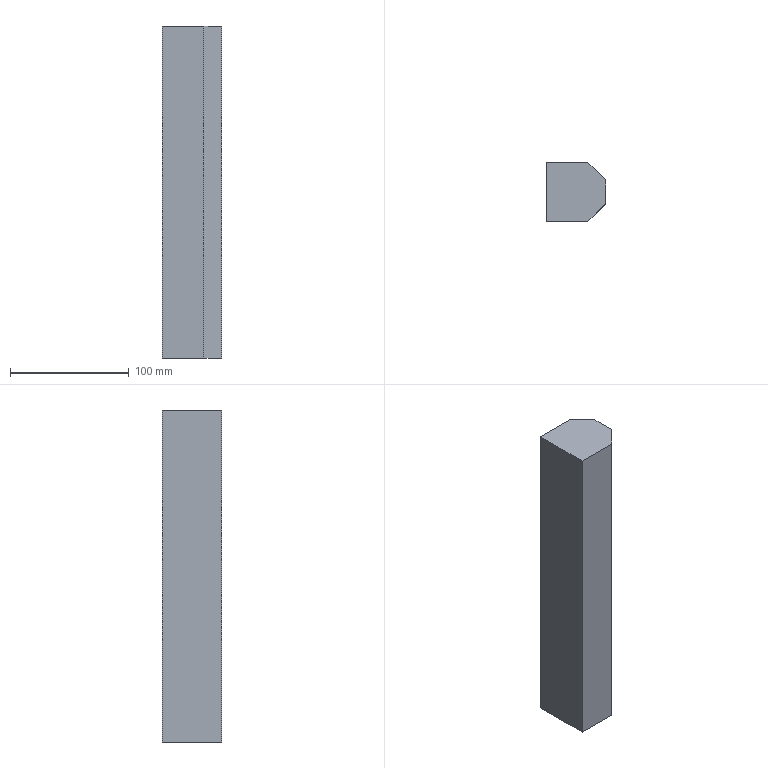Part | SolidWorks | features Chamfer 1, Extrusion 1 | 1 solid | 8 faces | box 50 x 50 x 280 mm | volume 637000 mm3 | plane 8
STEP:
#1=CARTESIAN_POINT('',(10.,-25.,140.));
#2=VERTEX_POINT('',#1);
#3=CARTESIAN_POINT('',(-25.,-25.,140.));
#4=VERTEX_POINT('',#3);
#5=CARTESIAN_POINT('',(25.,-25.,140.));
#6=DIRECTION('',(-1.,0.,0.));
#7=VECTOR('',#6,1000.);
#8=LINE('',#5,#7);
#9=EDGE_CURVE('',#2,#4,#8,.T.);
#10=ORIENTED_EDGE('',*,*,#9,.F.);
#11=CARTESIAN_POINT('',(25.,-10.,140.));
#12=VERTEX_POINT('',#11);
#13=CARTESIAN_POINT('',(25.,-10.,140.));
#14=DIRECTION('',(0.7071,0.7071,0.));
#15=VECTOR('',#14,1000.);
#16=LINE('',#13,#15);
#17=EDGE_CURVE('',#2,#12,#16,.T.);
#18=ORIENTED_EDGE('',*,*,#17,.T.);
#19=CARTESIAN_POINT('',(25.,10.,140.));
#20=VERTEX_POINT('',#19);
#21=CARTESIAN_POINT('',(25.,-25.,140.));
#22=DIRECTION('',(0.,-1.,0.));
#23=VECTOR('',#22,1000.);
#24=LINE('',#21,#23);
#25=EDGE_CURVE('',#20,#12,#24,.T.);
#26=ORIENTED_EDGE('',*,*,#25,.F.);
#27=CARTESIAN_POINT('',(10.,25.,140.));
#28=VERTEX_POINT('',#27);
#29=CARTESIAN_POINT('',(25.,10.,140.));
#30=DIRECTION('',(-0.7071,0.7071,0.));
#31=VECTOR('',#30,1000.);
#32=LINE('',#29,#31);
#33=EDGE_CURVE('',#20,#28,#32,.T.);
#34=ORIENTED_EDGE('',*,*,#33,.T.);
#35=CARTESIAN_POINT('',(-25.,25.,140.));
#36=VERTEX_POINT('',#35);
#37=CARTESIAN_POINT('',(25.,25.,140.));
#38=DIRECTION('',(-1.,0.,0.));
#39=VECTOR('',#38,1000.);
#40=LINE('',#37,#39);
#41=EDGE_CURVE('',#28,#36,#40,.T.);
#42=ORIENTED_EDGE('',*,*,#41,.T.);
#43=CARTESIAN_POINT('',(-25.,-25.,140.));
#44=DIRECTION('',(0.,-1.,0.));
#45=VECTOR('',#44,1000.);
#46=LINE('',#43,#45);
#47=EDGE_CURVE('',#36,#4,#46,.T.);
#48=ORIENTED_EDGE('',*,*,#47,.T.);
#49=EDGE_LOOP('',(#10,#18,#26,#34,#42,#48));
#50=FACE_OUTER_BOUND('',#49,.T.);
#51=CARTESIAN_POINT('',(25.,-25.,140.));
#52=DIRECTION('',(0.,0.,-1.));
#53=DIRECTION('',(-1.,0.,0.));
#54=AXIS2_PLACEMENT_3D('',#51,#52,#53);
#55=PLANE('',#54);
#56=ADVANCED_FACE('',(#50),#55,.F.);
#57=CARTESIAN_POINT('',(10.,-25.,-140.));
#58=VERTEX_POINT('',#57);
#59=CARTESIAN_POINT('',(-25.,-25.,-140.));
#60=VERTEX_POINT('',#59);
#61=CARTESIAN_POINT('',(25.,-25.,-140.));
#62=DIRECTION('',(-1.,0.,0.));
#63=VECTOR('',#62,1000.);
#64=LINE('',#61,#63);
#65=EDGE_CURVE('',#58,#60,#64,.T.);
#66=ORIENTED_EDGE('',*,*,#65,.F.);
#67=CARTESIAN_POINT('',(10.,-25.,140.));
#68=DIRECTION('',(0.,0.,1.));
#69=VECTOR('',#68,1000.);
#70=LINE('',#67,#69);
#71=EDGE_CURVE('',#58,#2,#70,.T.);
#72=ORIENTED_EDGE('',*,*,#71,.T.);
#73=ORIENTED_EDGE('',*,*,#9,.T.);
#74=CARTESIAN_POINT('',(-25.,-25.,-140.));
#75=DIRECTION('',(0.,0.,-1.));
#76=VECTOR('',#75,1000.);
#77=LINE('',#74,#76);
#78=EDGE_CURVE('',#4,#60,#77,.T.);
#79=ORIENTED_EDGE('',*,*,#78,.T.);
#80=EDGE_LOOP('',(#66,#72,#73,#79));
#81=FACE_OUTER_BOUND('',#80,.T.);
#82=CARTESIAN_POINT('',(25.,-25.,-140.));
#83=DIRECTION('',(0.,1.,0.));
#84=DIRECTION('',(0.,0.,1.));
#85=AXIS2_PLACEMENT_3D('',#82,#83,#84);
#86=PLANE('',#85);
#87=ADVANCED_FACE('',(#81),#86,.F.);
#88=CARTESIAN_POINT('',(25.,-10.,-140.));
#89=VERTEX_POINT('',#88);
#90=CARTESIAN_POINT('',(25.,10.,-140.));
#91=VERTEX_POINT('',#90);
#92=CARTESIAN_POINT('',(25.,-25.,-140.));
#93=DIRECTION('',(0.,1.,0.));
#94=VECTOR('',#93,1000.);
#95=LINE('',#92,#94);
#96=EDGE_CURVE('',#89,#91,#95,.T.);
#97=ORIENTED_EDGE('',*,*,#96,.F.);
#98=CARTESIAN_POINT('',(25.,-10.,-140.));
#99=DIRECTION('',(-0.7071,-0.7071,0.));
#100=VECTOR('',#99,1000.);
#101=LINE('',#98,#100);
#102=EDGE_CURVE('',#89,#58,#101,.T.);
#103=ORIENTED_EDGE('',*,*,#102,.T.);
#104=ORIENTED_EDGE('',*,*,#65,.T.);
#105=CARTESIAN_POINT('',(-25.,25.,-140.));
#106=VERTEX_POINT('',#105);
#107=CARTESIAN_POINT('',(-25.,-25.,-140.));
#108=DIRECTION('',(0.,1.,0.));
#109=VECTOR('',#108,1000.);
#110=LINE('',#107,#109);
#111=EDGE_CURVE('',#60,#106,#110,.T.);
#112=ORIENTED_EDGE('',*,*,#111,.T.);
#113=CARTESIAN_POINT('',(10.,25.,-140.));
#114=VERTEX_POINT('',#113);
#115=CARTESIAN_POINT('',(25.,25.,-140.));
#116=DIRECTION('',(-1.,0.,0.));
#117=VECTOR('',#116,1000.);
#118=LINE('',#115,#117);
#119=EDGE_CURVE('',#114,#106,#118,.T.);
#120=ORIENTED_EDGE('',*,*,#119,.F.);
#121=CARTESIAN_POINT('',(25.,10.,-140.));
#122=DIRECTION('',(0.7071,-0.7071,0.));
#123=VECTOR('',#122,1000.);
#124=LINE('',#121,#123);
#125=EDGE_CURVE('',#114,#91,#124,.T.);
#126=ORIENTED_EDGE('',*,*,#125,.T.);
#127=EDGE_LOOP('',(#97,#103,#104,#112,#120,#126));
#128=FACE_OUTER_BOUND('',#127,.T.);
#129=CARTESIAN_POINT('',(25.,-25.,-140.));
#130=DIRECTION('',(0.,0.,1.));
#131=DIRECTION('',(1.,0.,0.));
#132=AXIS2_PLACEMENT_3D('',#129,#130,#131);
#133=PLANE('',#132);
#134=ADVANCED_FACE('',(#128),#133,.F.);
#135=ORIENTED_EDGE('',*,*,#41,.F.);
#136=CARTESIAN_POINT('',(10.,25.,-140.));
#137=DIRECTION('',(0.,0.,-1.));
#138=VECTOR('',#137,1000.);
#139=LINE('',#136,#138);
#140=EDGE_CURVE('',#28,#114,#139,.T.);
#141=ORIENTED_EDGE('',*,*,#140,.T.);
#142=ORIENTED_EDGE('',*,*,#119,.T.);
#143=CARTESIAN_POINT('',(-25.,25.,-140.));
#144=DIRECTION('',(0.,0.,1.));
#145=VECTOR('',#144,1000.);
#146=LINE('',#143,#145);
#147=EDGE_CURVE('',#106,#36,#146,.T.);
#148=ORIENTED_EDGE('',*,*,#147,.T.);
#149=EDGE_LOOP('',(#135,#141,#142,#148));
#150=FACE_OUTER_BOUND('',#149,.T.);
#151=CARTESIAN_POINT('',(25.,25.,-140.));
#152=DIRECTION('',(0.,-1.,0.));
#153=DIRECTION('',(0.,0.,-1.));
#154=AXIS2_PLACEMENT_3D('',#151,#152,#153);
#155=PLANE('',#154);
#156=ADVANCED_FACE('',(#150),#155,.F.);
#157=ORIENTED_EDGE('',*,*,#25,.T.);
#158=CARTESIAN_POINT('',(25.,-10.,-140.));
#159=DIRECTION('',(0.,0.,-1.));
#160=VECTOR('',#159,1000.);
#161=LINE('',#158,#160);
#162=EDGE_CURVE('',#12,#89,#161,.T.);
#163=ORIENTED_EDGE('',*,*,#162,.T.);
#164=ORIENTED_EDGE('',*,*,#96,.T.);
#165=CARTESIAN_POINT('',(25.,10.,140.));
#166=DIRECTION('',(0.,0.,1.));
#167=VECTOR('',#166,1000.);
#168=LINE('',#165,#167);
#169=EDGE_CURVE('',#91,#20,#168,.T.);
#170=ORIENTED_EDGE('',*,*,#169,.T.);
#171=EDGE_LOOP('',(#157,#163,#164,#170));
#172=FACE_OUTER_BOUND('',#171,.T.);
#173=CARTESIAN_POINT('',(25.,0.,0.));
#174=DIRECTION('',(1.,0.,0.));
#175=DIRECTION('',(0.,0.,-1.));
#176=AXIS2_PLACEMENT_3D('',#173,#174,#175);
#177=PLANE('',#176);
#178=ADVANCED_FACE('',(#172),#177,.T.);
#179=ORIENTED_EDGE('',*,*,#47,.F.);
#180=ORIENTED_EDGE('',*,*,#147,.F.);
#181=ORIENTED_EDGE('',*,*,#111,.F.);
#182=ORIENTED_EDGE('',*,*,#78,.F.);
#183=EDGE_LOOP('',(#179,#180,#181,#182));
#184=FACE_OUTER_BOUND('',#183,.T.);
#185=CARTESIAN_POINT('',(-25.,0.,0.));
#186=DIRECTION('',(1.,0.,0.));
#187=DIRECTION('',(0.,0.,-1.));
#188=AXIS2_PLACEMENT_3D('',#185,#186,#187);
#189=PLANE('',#188);
#190=ADVANCED_FACE('',(#184),#189,.F.);
#191=ORIENTED_EDGE('',*,*,#17,.F.);
#192=ORIENTED_EDGE('',*,*,#71,.F.);
#193=ORIENTED_EDGE('',*,*,#102,.F.);
#194=ORIENTED_EDGE('',*,*,#162,.F.);
#195=EDGE_LOOP('',(#191,#192,#193,#194));
#196=FACE_OUTER_BOUND('',#195,.T.);
#197=CARTESIAN_POINT('',(25.,-10.,0.));
#198=DIRECTION('',(0.7071,-0.7071,0.));
#199=DIRECTION('',(0.,0.,1.));
#200=AXIS2_PLACEMENT_3D('',#197,#198,#199);
#201=PLANE('',#200);
#202=ADVANCED_FACE('',(#196),#201,.T.);
#203=ORIENTED_EDGE('',*,*,#125,.F.);
#204=ORIENTED_EDGE('',*,*,#140,.F.);
#205=ORIENTED_EDGE('',*,*,#33,.F.);
#206=ORIENTED_EDGE('',*,*,#169,.F.);
#207=EDGE_LOOP('',(#203,#204,#205,#206));
#208=FACE_OUTER_BOUND('',#207,.T.);
#209=CARTESIAN_POINT('',(25.,10.,0.));
#210=DIRECTION('',(0.7071,0.7071,0.));
#211=DIRECTION('',(0.,0.,-1.));
#212=AXIS2_PLACEMENT_3D('',#209,#210,#211);
#213=PLANE('',#212);
#214=ADVANCED_FACE('',(#208),#213,.T.);
#215=CLOSED_SHELL('',(#56,#87,#134,#156,#178,#190,#202,#214));
#216=MANIFOLD_SOLID_BREP('',#215);
#217=CARTESIAN_POINT('',(0.,0.,0.));
#218=DIRECTION('',(0.,0.,1.));
#219=DIRECTION('',(1.,0.,0.));
#220=AXIS2_PLACEMENT_3D('',#217,#218,#219);
#221=(LENGTH_UNIT()NAMED_UNIT(*)SI_UNIT(.MILLI.,.METRE.));
#222=UNCERTAINTY_MEASURE_WITH_UNIT(LENGTH_MEASURE(0.00001),#221,'','');
#223=(NAMED_UNIT(*)PLANE_ANGLE_UNIT()SI_UNIT($,.RADIAN.));
#224=(NAMED_UNIT(*)SI_UNIT($,.STERADIAN.)SOLID_ANGLE_UNIT());
#225=(GEOMETRIC_REPRESENTATION_CONTEXT(3)GLOBAL_UNCERTAINTY_ASSIGNED_CONTEXT((#222))GLOBAL_UNIT_ASSIGNED_CONTEXT((#221,#223,#224))REPRESENTATION_CONTEXT('',''));
#226=ADVANCED_BREP_SHAPE_REPRESENTATION('',(#216,#220),#225);